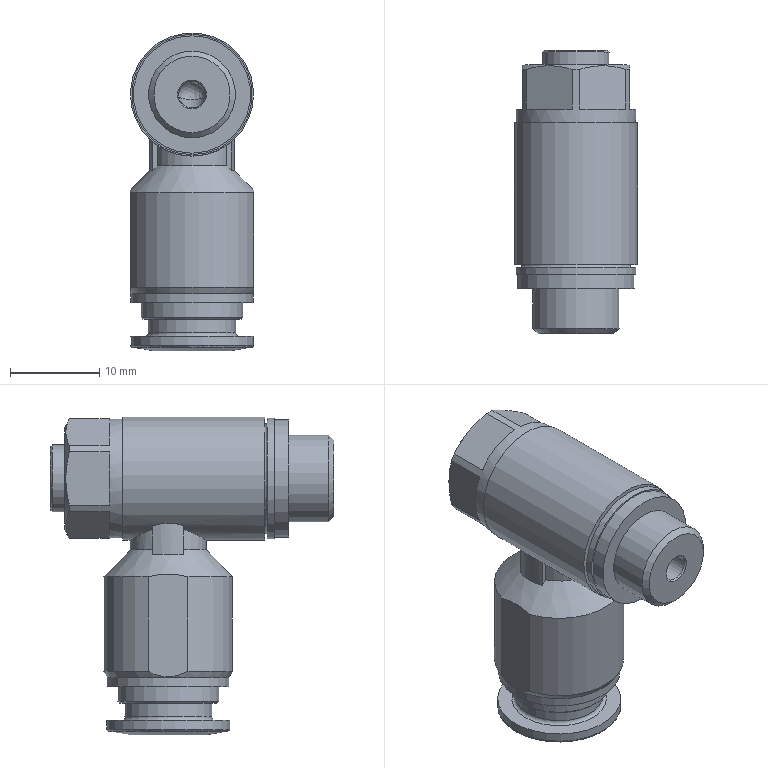Part | NX | features BREP 1 | 1 solid | 73 faces | box 13.8 x 31.75 x 35.6 mm | volume 5787 mm3 | plane 37 | cylinder 21 | cone 10 | torus 4 | sphere 1 | commonest cylinder face diameters 3 x3 8.5 x2 9.5 x2 13.8 x2 14.5 x2 6.3 x1